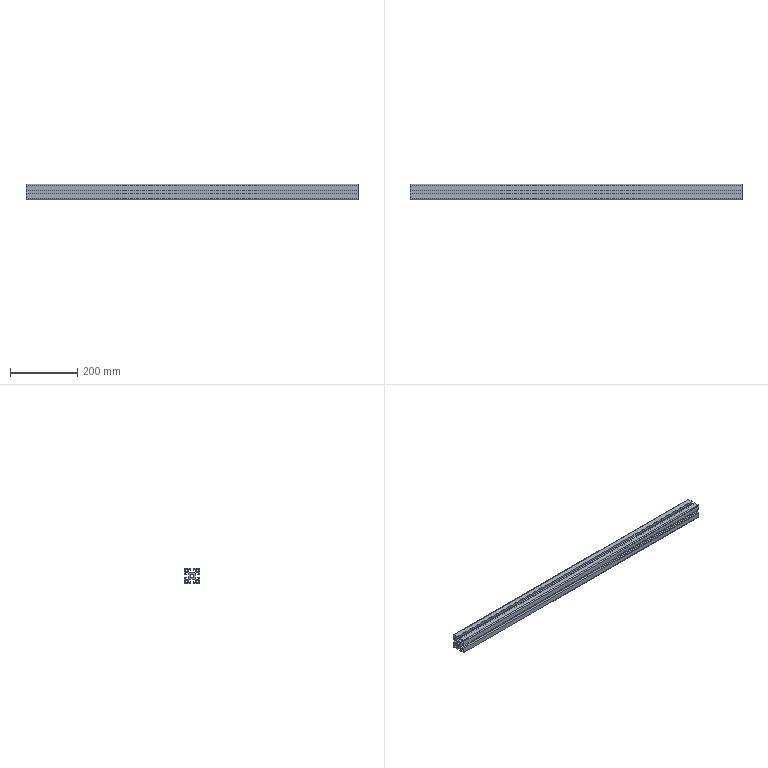Part | STEP file | 1_12 | 1 solid | 87 faces | box 985 x 45 x 45 mm | volume 805477 mm3 | plane 78 | cylinder 9 | commonest cylinder face diameters 2 x4 6 x4 10 x1